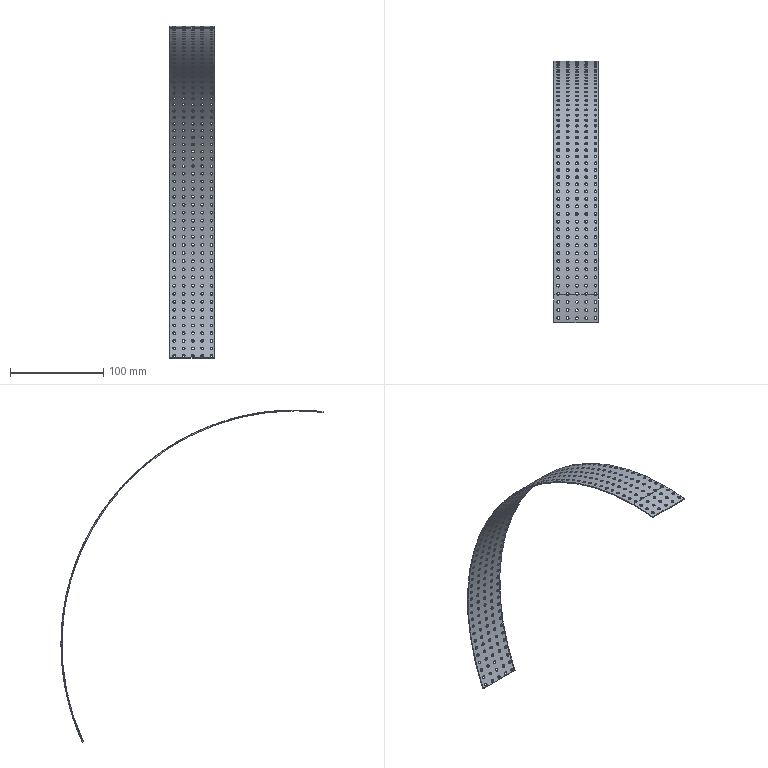Part | STEP file | 09-14 Track outer side plate | 1 solid | 618 faces | box 48 x 281 x 356 mm | volume 23365 mm3 | cylinder 614 | plane 4 | commonest cylinder face diameters 3 x610 500 x2 502 x2